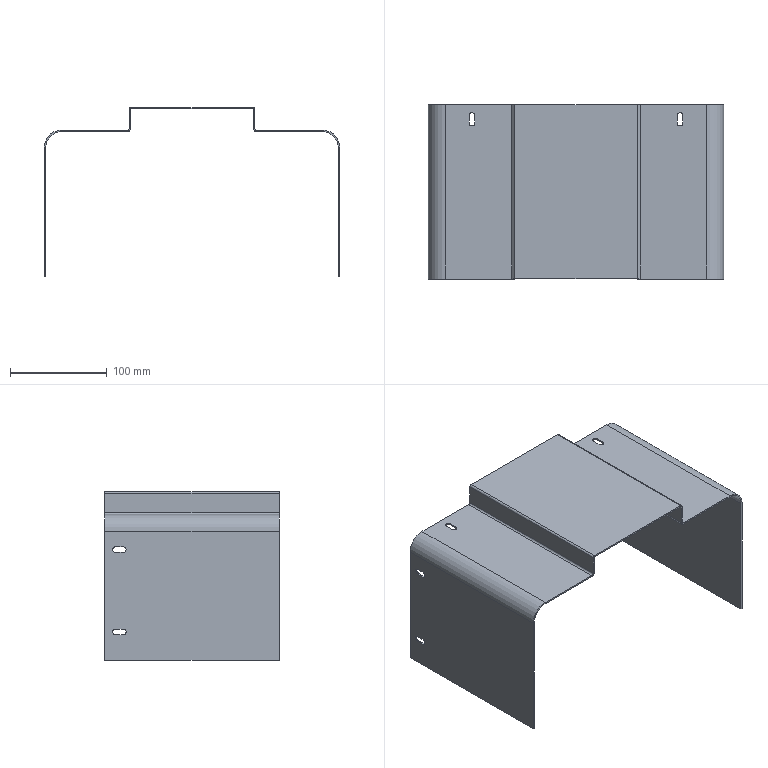Part | SolidWorks | features Fillet 2, HoleWzd 2, Shell 2, Extrusion 1, ICE 1 | 1 solid | 54 faces | box 305 x 180 x 174.5 mm | volume 170426 mm3 | plane 30 | cylinder 24 | commonest cylinder face diameters 5.8 x12 3.48 x4 0.48 x2 6.48 x2 32 x2 35 x2